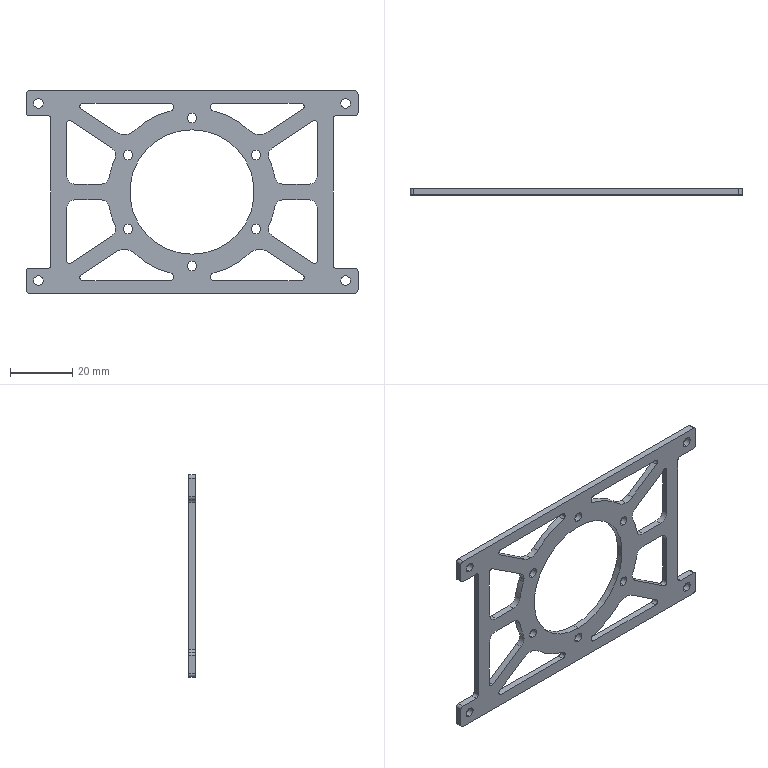Part | SolidWorks | features Fillet 3, Extrusion 1 | 1 solid | 116 faces | box 106.727 x 2 x 65 mm | volume 6307 mm3 | cylinder 78 | plane 38 | commonest cylinder face diameters 2 x30 3.1 x20 6 x12 54 x8 10 x6 40 x2